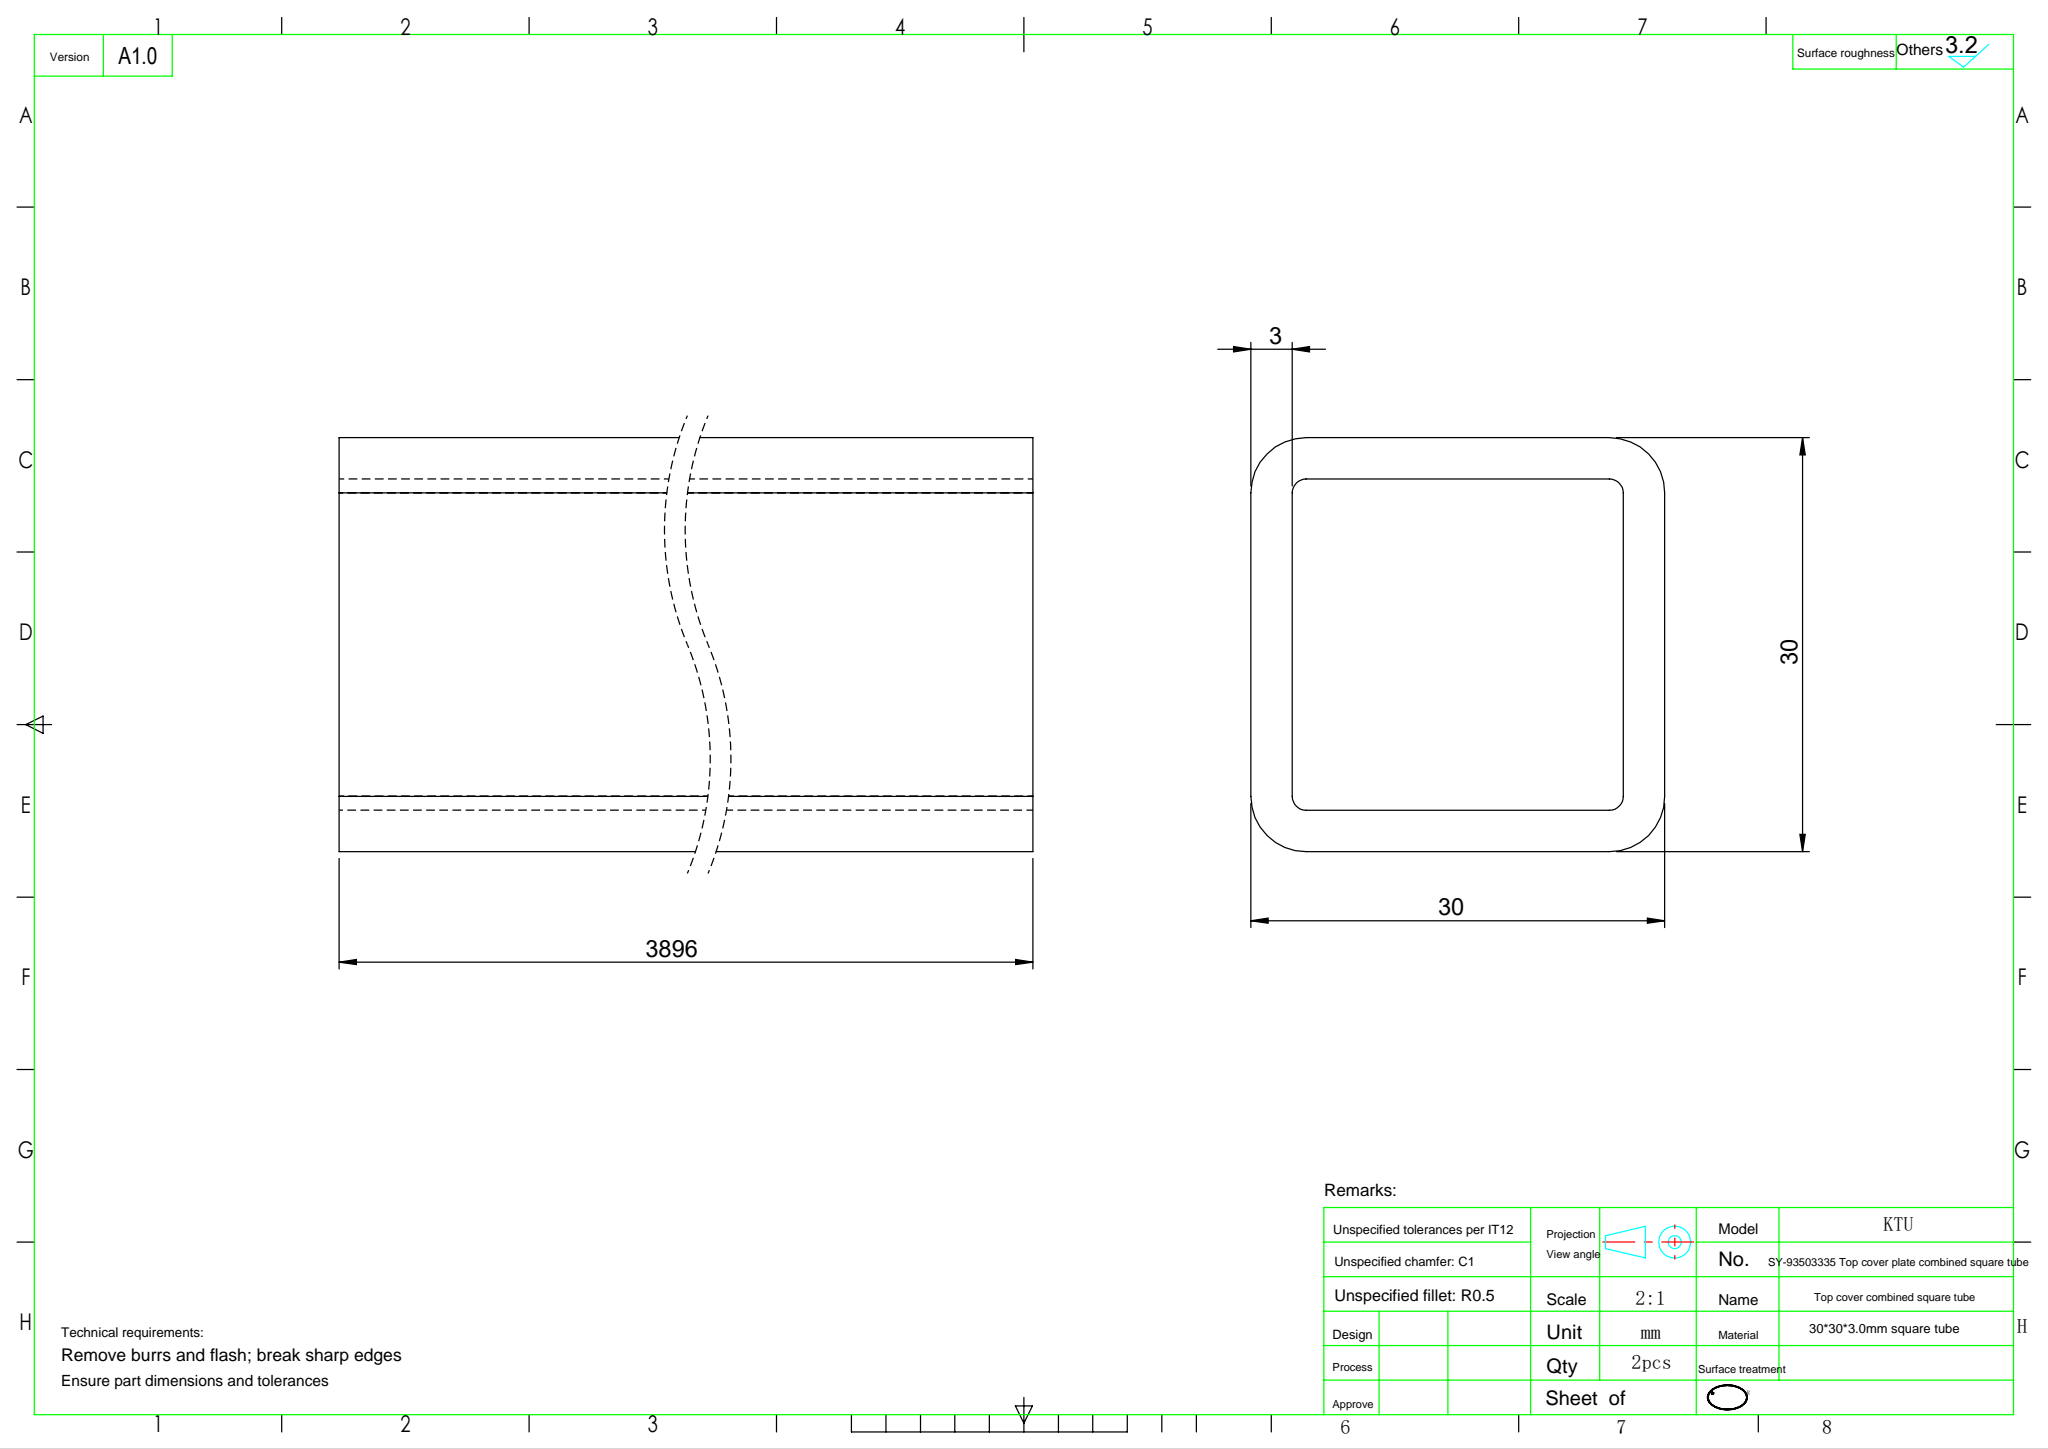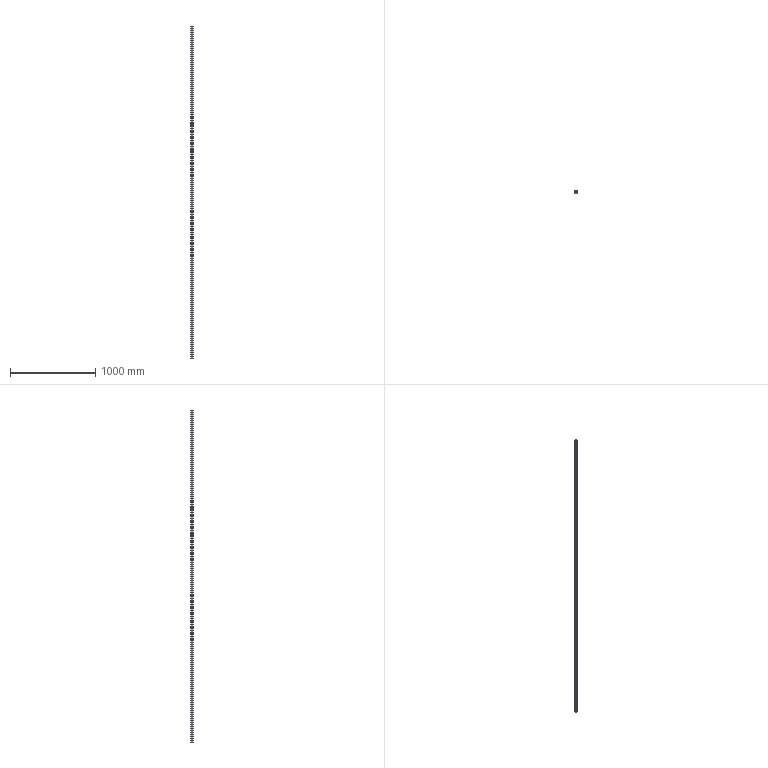Part | SolidWorks | features ExtruThin 1 | 1 solid | 18 faces | box 30 x 30 x 3896 mm | volume 1212139 mm3 | plane 10 | cylinder 8 | commonest cylinder face diameters 2 x4 8 x4
STEP:
#1=CARTESIAN_POINT('',(15.,11.,1948.));
#2=VERTEX_POINT('',#1);
#3=CARTESIAN_POINT('',(11.,15.,1948.));
#4=VERTEX_POINT('',#3);
#5=CARTESIAN_POINT('',(11.,11.,1948.));
#6=DIRECTION('',(0.,0.,1.));
#7=DIRECTION('',(-1.,0.,0.));
#8=AXIS2_PLACEMENT_3D('',#5,#6,#7);
#9=CIRCLE('',#8,4.);
#10=EDGE_CURVE('',#2,#4,#9,.T.);
#11=ORIENTED_EDGE('',*,*,#10,.T.);
#12=CARTESIAN_POINT('',(-11.,15.,1948.));
#13=VERTEX_POINT('',#12);
#14=CARTESIAN_POINT('',(-11.,15.,1948.));
#15=DIRECTION('',(-1.,0.,0.));
#16=VECTOR('',#15,1000.);
#17=LINE('',#14,#16);
#18=EDGE_CURVE('',#4,#13,#17,.T.);
#19=ORIENTED_EDGE('',*,*,#18,.T.);
#20=CARTESIAN_POINT('',(-15.,11.,1948.));
#21=VERTEX_POINT('',#20);
#22=CARTESIAN_POINT('',(-11.,11.,1948.));
#23=DIRECTION('',(0.,0.,1.));
#24=DIRECTION('',(1.,0.,0.));
#25=AXIS2_PLACEMENT_3D('',#22,#23,#24);
#26=CIRCLE('',#25,4.);
#27=EDGE_CURVE('',#13,#21,#26,.T.);
#28=ORIENTED_EDGE('',*,*,#27,.T.);
#29=CARTESIAN_POINT('',(-15.,-11.,1948.));
#30=VERTEX_POINT('',#29);
#31=CARTESIAN_POINT('',(-15.,11.,1948.));
#32=DIRECTION('',(0.,-1.,0.));
#33=VECTOR('',#32,1000.);
#34=LINE('',#31,#33);
#35=EDGE_CURVE('',#21,#30,#34,.T.);
#36=ORIENTED_EDGE('',*,*,#35,.T.);
#37=CARTESIAN_POINT('',(-11.,-15.,1948.));
#38=VERTEX_POINT('',#37);
#39=CARTESIAN_POINT('',(-11.,-11.,1948.));
#40=DIRECTION('',(0.,0.,1.));
#41=DIRECTION('',(1.,0.,0.));
#42=AXIS2_PLACEMENT_3D('',#39,#40,#41);
#43=CIRCLE('',#42,4.);
#44=EDGE_CURVE('',#30,#38,#43,.T.);
#45=ORIENTED_EDGE('',*,*,#44,.T.);
#46=CARTESIAN_POINT('',(11.,-15.,1948.));
#47=VERTEX_POINT('',#46);
#48=CARTESIAN_POINT('',(-11.,-15.,1948.));
#49=DIRECTION('',(1.,0.,0.));
#50=VECTOR('',#49,1000.);
#51=LINE('',#48,#50);
#52=EDGE_CURVE('',#38,#47,#51,.T.);
#53=ORIENTED_EDGE('',*,*,#52,.T.);
#54=CARTESIAN_POINT('',(15.,-11.,1948.));
#55=VERTEX_POINT('',#54);
#56=CARTESIAN_POINT('',(11.,-11.,1948.));
#57=DIRECTION('',(0.,0.,1.));
#58=DIRECTION('',(1.,0.,0.));
#59=AXIS2_PLACEMENT_3D('',#56,#57,#58);
#60=CIRCLE('',#59,4.);
#61=EDGE_CURVE('',#47,#55,#60,.T.);
#62=ORIENTED_EDGE('',*,*,#61,.T.);
#63=CARTESIAN_POINT('',(15.,11.,1948.));
#64=DIRECTION('',(0.,1.,0.));
#65=VECTOR('',#64,1000.);
#66=LINE('',#63,#65);
#67=EDGE_CURVE('',#55,#2,#66,.T.);
#68=ORIENTED_EDGE('',*,*,#67,.T.);
#69=EDGE_LOOP('',(#11,#19,#28,#36,#45,#53,#62,#68));
#70=FACE_OUTER_BOUND('',#69,.T.);
#71=CARTESIAN_POINT('',(11.,12.,1948.));
#72=VERTEX_POINT('',#71);
#73=CARTESIAN_POINT('',(-11.,12.,1948.));
#74=VERTEX_POINT('',#73);
#75=CARTESIAN_POINT('',(11.,12.,1948.));
#76=DIRECTION('',(-1.,0.,0.));
#77=VECTOR('',#76,1000.);
#78=LINE('',#75,#77);
#79=EDGE_CURVE('',#72,#74,#78,.T.);
#80=ORIENTED_EDGE('',*,*,#79,.F.);
#81=CARTESIAN_POINT('',(12.,11.,1948.));
#82=VERTEX_POINT('',#81);
#83=CARTESIAN_POINT('',(11.,11.,1948.));
#84=DIRECTION('',(0.,0.,1.));
#85=DIRECTION('',(-1.,0.,0.));
#86=AXIS2_PLACEMENT_3D('',#83,#84,#85);
#87=CIRCLE('',#86,1.);
#88=EDGE_CURVE('',#82,#72,#87,.T.);
#89=ORIENTED_EDGE('',*,*,#88,.F.);
#90=CARTESIAN_POINT('',(12.,-11.,1948.));
#91=VERTEX_POINT('',#90);
#92=CARTESIAN_POINT('',(12.,11.,1948.));
#93=DIRECTION('',(0.,1.,0.));
#94=VECTOR('',#93,1000.);
#95=LINE('',#92,#94);
#96=EDGE_CURVE('',#91,#82,#95,.T.);
#97=ORIENTED_EDGE('',*,*,#96,.F.);
#98=CARTESIAN_POINT('',(11.,-12.,1948.));
#99=VERTEX_POINT('',#98);
#100=CARTESIAN_POINT('',(11.,-11.,1948.));
#101=DIRECTION('',(0.,0.,1.));
#102=DIRECTION('',(-1.,0.,0.));
#103=AXIS2_PLACEMENT_3D('',#100,#101,#102);
#104=CIRCLE('',#103,1.);
#105=EDGE_CURVE('',#99,#91,#104,.T.);
#106=ORIENTED_EDGE('',*,*,#105,.F.);
#107=CARTESIAN_POINT('',(-11.,-12.,1948.));
#108=VERTEX_POINT('',#107);
#109=CARTESIAN_POINT('',(11.,-12.,1948.));
#110=DIRECTION('',(1.,0.,0.));
#111=VECTOR('',#110,1000.);
#112=LINE('',#109,#111);
#113=EDGE_CURVE('',#108,#99,#112,.T.);
#114=ORIENTED_EDGE('',*,*,#113,.F.);
#115=CARTESIAN_POINT('',(-12.,-11.,1948.));
#116=VERTEX_POINT('',#115);
#117=CARTESIAN_POINT('',(-11.,-11.,1948.));
#118=DIRECTION('',(0.,0.,1.));
#119=DIRECTION('',(-1.,0.,0.));
#120=AXIS2_PLACEMENT_3D('',#117,#118,#119);
#121=CIRCLE('',#120,1.);
#122=EDGE_CURVE('',#116,#108,#121,.T.);
#123=ORIENTED_EDGE('',*,*,#122,.F.);
#124=CARTESIAN_POINT('',(-12.,11.,1948.));
#125=VERTEX_POINT('',#124);
#126=CARTESIAN_POINT('',(-12.,11.,1948.));
#127=DIRECTION('',(0.,-1.,0.));
#128=VECTOR('',#127,1000.);
#129=LINE('',#126,#128);
#130=EDGE_CURVE('',#125,#116,#129,.T.);
#131=ORIENTED_EDGE('',*,*,#130,.F.);
#132=CARTESIAN_POINT('',(-11.,11.,1948.));
#133=DIRECTION('',(0.,0.,1.));
#134=DIRECTION('',(-1.,0.,0.));
#135=AXIS2_PLACEMENT_3D('',#132,#133,#134);
#136=CIRCLE('',#135,1.);
#137=EDGE_CURVE('',#74,#125,#136,.T.);
#138=ORIENTED_EDGE('',*,*,#137,.F.);
#139=EDGE_LOOP('',(#80,#89,#97,#106,#114,#123,#131,#138));
#140=FACE_BOUND('',#139,.T.);
#141=CARTESIAN_POINT('',(11.,11.,1948.));
#142=DIRECTION('',(0.,0.,1.));
#143=DIRECTION('',(1.,0.,0.));
#144=AXIS2_PLACEMENT_3D('',#141,#142,#143);
#145=PLANE('',#144);
#146=ADVANCED_FACE('',(#70,#140),#145,.T.);
#147=CARTESIAN_POINT('',(15.,11.,-1948.));
#148=VERTEX_POINT('',#147);
#149=CARTESIAN_POINT('',(11.,15.,-1948.));
#150=VERTEX_POINT('',#149);
#151=CARTESIAN_POINT('',(11.,11.,-1948.));
#152=DIRECTION('',(0.,0.,1.));
#153=DIRECTION('',(-1.,0.,0.));
#154=AXIS2_PLACEMENT_3D('',#151,#152,#153);
#155=CIRCLE('',#154,4.);
#156=EDGE_CURVE('',#148,#150,#155,.T.);
#157=ORIENTED_EDGE('',*,*,#156,.F.);
#158=CARTESIAN_POINT('',(15.,-11.,-1948.));
#159=VERTEX_POINT('',#158);
#160=CARTESIAN_POINT('',(15.,11.,-1948.));
#161=DIRECTION('',(0.,1.,0.));
#162=VECTOR('',#161,1000.);
#163=LINE('',#160,#162);
#164=EDGE_CURVE('',#159,#148,#163,.T.);
#165=ORIENTED_EDGE('',*,*,#164,.F.);
#166=CARTESIAN_POINT('',(11.,-15.,-1948.));
#167=VERTEX_POINT('',#166);
#168=CARTESIAN_POINT('',(11.,-11.,-1948.));
#169=DIRECTION('',(0.,0.,1.));
#170=DIRECTION('',(1.,0.,0.));
#171=AXIS2_PLACEMENT_3D('',#168,#169,#170);
#172=CIRCLE('',#171,4.);
#173=EDGE_CURVE('',#167,#159,#172,.T.);
#174=ORIENTED_EDGE('',*,*,#173,.F.);
#175=CARTESIAN_POINT('',(-11.,-15.,-1948.));
#176=VERTEX_POINT('',#175);
#177=CARTESIAN_POINT('',(-11.,-15.,-1948.));
#178=DIRECTION('',(1.,0.,0.));
#179=VECTOR('',#178,1000.);
#180=LINE('',#177,#179);
#181=EDGE_CURVE('',#176,#167,#180,.T.);
#182=ORIENTED_EDGE('',*,*,#181,.F.);
#183=CARTESIAN_POINT('',(-15.,-11.,-1948.));
#184=VERTEX_POINT('',#183);
#185=CARTESIAN_POINT('',(-11.,-11.,-1948.));
#186=DIRECTION('',(0.,0.,1.));
#187=DIRECTION('',(1.,0.,0.));
#188=AXIS2_PLACEMENT_3D('',#185,#186,#187);
#189=CIRCLE('',#188,4.);
#190=EDGE_CURVE('',#184,#176,#189,.T.);
#191=ORIENTED_EDGE('',*,*,#190,.F.);
#192=CARTESIAN_POINT('',(-15.,11.,-1948.));
#193=VERTEX_POINT('',#192);
#194=CARTESIAN_POINT('',(-15.,11.,-1948.));
#195=DIRECTION('',(0.,-1.,0.));
#196=VECTOR('',#195,1000.);
#197=LINE('',#194,#196);
#198=EDGE_CURVE('',#193,#184,#197,.T.);
#199=ORIENTED_EDGE('',*,*,#198,.F.);
#200=CARTESIAN_POINT('',(-11.,15.,-1948.));
#201=VERTEX_POINT('',#200);
#202=CARTESIAN_POINT('',(-11.,11.,-1948.));
#203=DIRECTION('',(0.,0.,1.));
#204=DIRECTION('',(1.,0.,0.));
#205=AXIS2_PLACEMENT_3D('',#202,#203,#204);
#206=CIRCLE('',#205,4.);
#207=EDGE_CURVE('',#201,#193,#206,.T.);
#208=ORIENTED_EDGE('',*,*,#207,.F.);
#209=CARTESIAN_POINT('',(-11.,15.,-1948.));
#210=DIRECTION('',(-1.,0.,0.));
#211=VECTOR('',#210,1000.);
#212=LINE('',#209,#211);
#213=EDGE_CURVE('',#150,#201,#212,.T.);
#214=ORIENTED_EDGE('',*,*,#213,.F.);
#215=EDGE_LOOP('',(#157,#165,#174,#182,#191,#199,#208,#214));
#216=FACE_OUTER_BOUND('',#215,.T.);
#217=CARTESIAN_POINT('',(12.,11.,-1948.));
#218=VERTEX_POINT('',#217);
#219=CARTESIAN_POINT('',(11.,12.,-1948.));
#220=VERTEX_POINT('',#219);
#221=CARTESIAN_POINT('',(11.,11.,-1948.));
#222=DIRECTION('',(0.,0.,1.));
#223=DIRECTION('',(-1.,0.,0.));
#224=AXIS2_PLACEMENT_3D('',#221,#222,#223);
#225=CIRCLE('',#224,1.);
#226=EDGE_CURVE('',#218,#220,#225,.T.);
#227=ORIENTED_EDGE('',*,*,#226,.T.);
#228=CARTESIAN_POINT('',(-11.,12.,-1948.));
#229=VERTEX_POINT('',#228);
#230=CARTESIAN_POINT('',(11.,12.,-1948.));
#231=DIRECTION('',(-1.,0.,0.));
#232=VECTOR('',#231,1000.);
#233=LINE('',#230,#232);
#234=EDGE_CURVE('',#220,#229,#233,.T.);
#235=ORIENTED_EDGE('',*,*,#234,.T.);
#236=CARTESIAN_POINT('',(-12.,11.,-1948.));
#237=VERTEX_POINT('',#236);
#238=CARTESIAN_POINT('',(-11.,11.,-1948.));
#239=DIRECTION('',(0.,0.,1.));
#240=DIRECTION('',(-1.,0.,0.));
#241=AXIS2_PLACEMENT_3D('',#238,#239,#240);
#242=CIRCLE('',#241,1.);
#243=EDGE_CURVE('',#229,#237,#242,.T.);
#244=ORIENTED_EDGE('',*,*,#243,.T.);
#245=CARTESIAN_POINT('',(-12.,-11.,-1948.));
#246=VERTEX_POINT('',#245);
#247=CARTESIAN_POINT('',(-12.,11.,-1948.));
#248=DIRECTION('',(0.,-1.,0.));
#249=VECTOR('',#248,1000.);
#250=LINE('',#247,#249);
#251=EDGE_CURVE('',#237,#246,#250,.T.);
#252=ORIENTED_EDGE('',*,*,#251,.T.);
#253=CARTESIAN_POINT('',(-11.,-12.,-1948.));
#254=VERTEX_POINT('',#253);
#255=CARTESIAN_POINT('',(-11.,-11.,-1948.));
#256=DIRECTION('',(0.,0.,1.));
#257=DIRECTION('',(-1.,0.,0.));
#258=AXIS2_PLACEMENT_3D('',#255,#256,#257);
#259=CIRCLE('',#258,1.);
#260=EDGE_CURVE('',#246,#254,#259,.T.);
#261=ORIENTED_EDGE('',*,*,#260,.T.);
#262=CARTESIAN_POINT('',(11.,-12.,-1948.));
#263=VERTEX_POINT('',#262);
#264=CARTESIAN_POINT('',(11.,-12.,-1948.));
#265=DIRECTION('',(1.,0.,0.));
#266=VECTOR('',#265,1000.);
#267=LINE('',#264,#266);
#268=EDGE_CURVE('',#254,#263,#267,.T.);
#269=ORIENTED_EDGE('',*,*,#268,.T.);
#270=CARTESIAN_POINT('',(12.,-11.,-1948.));
#271=VERTEX_POINT('',#270);
#272=CARTESIAN_POINT('',(11.,-11.,-1948.));
#273=DIRECTION('',(0.,0.,1.));
#274=DIRECTION('',(-1.,0.,0.));
#275=AXIS2_PLACEMENT_3D('',#272,#273,#274);
#276=CIRCLE('',#275,1.);
#277=EDGE_CURVE('',#263,#271,#276,.T.);
#278=ORIENTED_EDGE('',*,*,#277,.T.);
#279=CARTESIAN_POINT('',(12.,11.,-1948.));
#280=DIRECTION('',(0.,1.,0.));
#281=VECTOR('',#280,1000.);
#282=LINE('',#279,#281);
#283=EDGE_CURVE('',#271,#218,#282,.T.);
#284=ORIENTED_EDGE('',*,*,#283,.T.);
#285=EDGE_LOOP('',(#227,#235,#244,#252,#261,#269,#278,#284));
#286=FACE_BOUND('',#285,.T.);
#287=CARTESIAN_POINT('',(11.,11.,-1948.));
#288=DIRECTION('',(0.,0.,1.));
#289=DIRECTION('',(1.,0.,0.));
#290=AXIS2_PLACEMENT_3D('',#287,#288,#289);
#291=PLANE('',#290);
#292=ADVANCED_FACE('',(#216,#286),#291,.F.);
#293=ORIENTED_EDGE('',*,*,#156,.T.);
#294=CARTESIAN_POINT('',(11.,15.,1948.));
#295=DIRECTION('',(0.,0.,-1.));
#296=VECTOR('',#295,1000.);
#297=LINE('',#294,#296);
#298=EDGE_CURVE('',#4,#150,#297,.T.);
#299=ORIENTED_EDGE('',*,*,#298,.F.);
#300=ORIENTED_EDGE('',*,*,#10,.F.);
#301=CARTESIAN_POINT('',(15.,11.,1948.));
#302=DIRECTION('',(0.,0.,-1.));
#303=VECTOR('',#302,1000.);
#304=LINE('',#301,#303);
#305=EDGE_CURVE('',#2,#148,#304,.T.);
#306=ORIENTED_EDGE('',*,*,#305,.T.);
#307=EDGE_LOOP('',(#293,#299,#300,#306));
#308=FACE_OUTER_BOUND('',#307,.T.);
#309=CARTESIAN_POINT('',(11.,11.,1948.));
#310=DIRECTION('',(0.,0.,-1.));
#311=DIRECTION('',(-1.,0.,0.));
#312=AXIS2_PLACEMENT_3D('',#309,#310,#311);
#313=CYLINDRICAL_SURFACE('',#312,4.);
#314=ADVANCED_FACE('',(#308),#313,.T.);
#315=ORIENTED_EDGE('',*,*,#213,.T.);
#316=CARTESIAN_POINT('',(-11.,15.,1948.));
#317=DIRECTION('',(0.,0.,-1.));
#318=VECTOR('',#317,1000.);
#319=LINE('',#316,#318);
#320=EDGE_CURVE('',#13,#201,#319,.T.);
#321=ORIENTED_EDGE('',*,*,#320,.F.);
#322=ORIENTED_EDGE('',*,*,#18,.F.);
#323=ORIENTED_EDGE('',*,*,#298,.T.);
#324=EDGE_LOOP('',(#315,#321,#322,#323));
#325=FACE_OUTER_BOUND('',#324,.T.);
#326=CARTESIAN_POINT('',(-11.,15.,1948.));
#327=DIRECTION('',(0.,-1.,0.));
#328=DIRECTION('',(0.,0.,-1.));
#329=AXIS2_PLACEMENT_3D('',#326,#327,#328);
#330=PLANE('',#329);
#331=ADVANCED_FACE('',(#325),#330,.F.);
#332=ORIENTED_EDGE('',*,*,#207,.T.);
#333=CARTESIAN_POINT('',(-15.,11.,1948.));
#334=DIRECTION('',(0.,0.,-1.));
#335=VECTOR('',#334,1000.);
#336=LINE('',#333,#335);
#337=EDGE_CURVE('',#21,#193,#336,.T.);
#338=ORIENTED_EDGE('',*,*,#337,.F.);
#339=ORIENTED_EDGE('',*,*,#27,.F.);
#340=ORIENTED_EDGE('',*,*,#320,.T.);
#341=EDGE_LOOP('',(#332,#338,#339,#340));
#342=FACE_OUTER_BOUND('',#341,.T.);
#343=CARTESIAN_POINT('',(-11.,11.,1948.));
#344=DIRECTION('',(0.,0.,-1.));
#345=DIRECTION('',(-1.,0.,0.));
#346=AXIS2_PLACEMENT_3D('',#343,#344,#345);
#347=CYLINDRICAL_SURFACE('',#346,4.);
#348=ADVANCED_FACE('',(#342),#347,.T.);
#349=ORIENTED_EDGE('',*,*,#198,.T.);
#350=CARTESIAN_POINT('',(-15.,-11.,1948.));
#351=DIRECTION('',(0.,0.,-1.));
#352=VECTOR('',#351,1000.);
#353=LINE('',#350,#352);
#354=EDGE_CURVE('',#30,#184,#353,.T.);
#355=ORIENTED_EDGE('',*,*,#354,.F.);
#356=ORIENTED_EDGE('',*,*,#35,.F.);
#357=ORIENTED_EDGE('',*,*,#337,.T.);
#358=EDGE_LOOP('',(#349,#355,#356,#357));
#359=FACE_OUTER_BOUND('',#358,.T.);
#360=CARTESIAN_POINT('',(-15.,11.,1948.));
#361=DIRECTION('',(1.,0.,0.));
#362=DIRECTION('',(0.,1.,0.));
#363=AXIS2_PLACEMENT_3D('',#360,#361,#362);
#364=PLANE('',#363);
#365=ADVANCED_FACE('',(#359),#364,.F.);
#366=ORIENTED_EDGE('',*,*,#190,.T.);
#367=CARTESIAN_POINT('',(-11.,-15.,1948.));
#368=DIRECTION('',(0.,0.,-1.));
#369=VECTOR('',#368,1000.);
#370=LINE('',#367,#369);
#371=EDGE_CURVE('',#38,#176,#370,.T.);
#372=ORIENTED_EDGE('',*,*,#371,.F.);
#373=ORIENTED_EDGE('',*,*,#44,.F.);
#374=ORIENTED_EDGE('',*,*,#354,.T.);
#375=EDGE_LOOP('',(#366,#372,#373,#374));
#376=FACE_OUTER_BOUND('',#375,.T.);
#377=CARTESIAN_POINT('',(-11.,-11.,1948.));
#378=DIRECTION('',(0.,0.,-1.));
#379=DIRECTION('',(-1.,0.,0.));
#380=AXIS2_PLACEMENT_3D('',#377,#378,#379);
#381=CYLINDRICAL_SURFACE('',#380,4.);
#382=ADVANCED_FACE('',(#376),#381,.T.);
#383=ORIENTED_EDGE('',*,*,#181,.T.);
#384=CARTESIAN_POINT('',(11.,-15.,1948.));
#385=DIRECTION('',(0.,0.,-1.));
#386=VECTOR('',#385,1000.);
#387=LINE('',#384,#386);
#388=EDGE_CURVE('',#47,#167,#387,.T.);
#389=ORIENTED_EDGE('',*,*,#388,.F.);
#390=ORIENTED_EDGE('',*,*,#52,.F.);
#391=ORIENTED_EDGE('',*,*,#371,.T.);
#392=EDGE_LOOP('',(#383,#389,#390,#391));
#393=FACE_OUTER_BOUND('',#392,.T.);
#394=CARTESIAN_POINT('',(-11.,-15.,1948.));
#395=DIRECTION('',(0.,1.,0.));
#396=DIRECTION('',(0.,0.,1.));
#397=AXIS2_PLACEMENT_3D('',#394,#395,#396);
#398=PLANE('',#397);
#399=ADVANCED_FACE('',(#393),#398,.F.);
#400=ORIENTED_EDGE('',*,*,#173,.T.);
#401=CARTESIAN_POINT('',(15.,-11.,1948.));
#402=DIRECTION('',(0.,0.,-1.));
#403=VECTOR('',#402,1000.);
#404=LINE('',#401,#403);
#405=EDGE_CURVE('',#55,#159,#404,.T.);
#406=ORIENTED_EDGE('',*,*,#405,.F.);
#407=ORIENTED_EDGE('',*,*,#61,.F.);
#408=ORIENTED_EDGE('',*,*,#388,.T.);
#409=EDGE_LOOP('',(#400,#406,#407,#408));
#410=FACE_OUTER_BOUND('',#409,.T.);
#411=CARTESIAN_POINT('',(11.,-11.,1948.));
#412=DIRECTION('',(0.,0.,-1.));
#413=DIRECTION('',(-1.,0.,0.));
#414=AXIS2_PLACEMENT_3D('',#411,#412,#413);
#415=CYLINDRICAL_SURFACE('',#414,4.);
#416=ADVANCED_FACE('',(#410),#415,.T.);
#417=ORIENTED_EDGE('',*,*,#164,.T.);
#418=ORIENTED_EDGE('',*,*,#305,.F.);
#419=ORIENTED_EDGE('',*,*,#67,.F.);
#420=ORIENTED_EDGE('',*,*,#405,.T.);
#421=EDGE_LOOP('',(#417,#418,#419,#420));
#422=FACE_OUTER_BOUND('',#421,.T.);
#423=CARTESIAN_POINT('',(15.,11.,1948.));
#424=DIRECTION('',(-1.,0.,0.));
#425=DIRECTION('',(0.,-1.,0.));
#426=AXIS2_PLACEMENT_3D('',#423,#424,#425);
#427=PLANE('',#426);
#428=ADVANCED_FACE('',(#422),#427,.F.);
#429=ORIENTED_EDGE('',*,*,#226,.F.);
#430=CARTESIAN_POINT('',(12.,11.,1948.));
#431=DIRECTION('',(0.,0.,-1.));
#432=VECTOR('',#431,1000.);
#433=LINE('',#430,#432);
#434=EDGE_CURVE('',#82,#218,#433,.T.);
#435=ORIENTED_EDGE('',*,*,#434,.F.);
#436=ORIENTED_EDGE('',*,*,#88,.T.);
#437=CARTESIAN_POINT('',(11.,12.,1948.));
#438=DIRECTION('',(0.,0.,-1.));
#439=VECTOR('',#438,1000.);
#440=LINE('',#437,#439);
#441=EDGE_CURVE('',#72,#220,#440,.T.);
#442=ORIENTED_EDGE('',*,*,#441,.T.);
#443=EDGE_LOOP('',(#429,#435,#436,#442));
#444=FACE_OUTER_BOUND('',#443,.T.);
#445=CARTESIAN_POINT('',(11.,11.,1948.));
#446=DIRECTION('',(0.,0.,-1.));
#447=DIRECTION('',(-1.,0.,0.));
#448=AXIS2_PLACEMENT_3D('',#445,#446,#447);
#449=CYLINDRICAL_SURFACE('',#448,1.);
#450=ADVANCED_FACE('',(#444),#449,.F.);
#451=ORIENTED_EDGE('',*,*,#234,.F.);
#452=ORIENTED_EDGE('',*,*,#441,.F.);
#453=ORIENTED_EDGE('',*,*,#79,.T.);
#454=CARTESIAN_POINT('',(-11.,12.,1948.));
#455=DIRECTION('',(0.,0.,-1.));
#456=VECTOR('',#455,1000.);
#457=LINE('',#454,#456);
#458=EDGE_CURVE('',#74,#229,#457,.T.);
#459=ORIENTED_EDGE('',*,*,#458,.T.);
#460=EDGE_LOOP('',(#451,#452,#453,#459));
#461=FACE_OUTER_BOUND('',#460,.T.);
#462=CARTESIAN_POINT('',(11.,12.,1948.));
#463=DIRECTION('',(0.,-1.,0.));
#464=DIRECTION('',(0.,0.,-1.));
#465=AXIS2_PLACEMENT_3D('',#462,#463,#464);
#466=PLANE('',#465);
#467=ADVANCED_FACE('',(#461),#466,.T.);
#468=ORIENTED_EDGE('',*,*,#243,.F.);
#469=ORIENTED_EDGE('',*,*,#458,.F.);
#470=ORIENTED_EDGE('',*,*,#137,.T.);
#471=CARTESIAN_POINT('',(-12.,11.,1948.));
#472=DIRECTION('',(0.,0.,-1.));
#473=VECTOR('',#472,1000.);
#474=LINE('',#471,#473);
#475=EDGE_CURVE('',#125,#237,#474,.T.);
#476=ORIENTED_EDGE('',*,*,#475,.T.);
#477=EDGE_LOOP('',(#468,#469,#470,#476));
#478=FACE_OUTER_BOUND('',#477,.T.);
#479=CARTESIAN_POINT('',(-11.,11.,1948.));
#480=DIRECTION('',(0.,0.,-1.));
#481=DIRECTION('',(-1.,0.,0.));
#482=AXIS2_PLACEMENT_3D('',#479,#480,#481);
#483=CYLINDRICAL_SURFACE('',#482,1.);
#484=ADVANCED_FACE('',(#478),#483,.F.);
#485=ORIENTED_EDGE('',*,*,#251,.F.);
#486=ORIENTED_EDGE('',*,*,#475,.F.);
#487=ORIENTED_EDGE('',*,*,#130,.T.);
#488=CARTESIAN_POINT('',(-12.,-11.,1948.));
#489=DIRECTION('',(0.,0.,-1.));
#490=VECTOR('',#489,1000.);
#491=LINE('',#488,#490);
#492=EDGE_CURVE('',#116,#246,#491,.T.);
#493=ORIENTED_EDGE('',*,*,#492,.T.);
#494=EDGE_LOOP('',(#485,#486,#487,#493));
#495=FACE_OUTER_BOUND('',#494,.T.);
#496=CARTESIAN_POINT('',(-12.,11.,1948.));
#497=DIRECTION('',(1.,0.,0.));
#498=DIRECTION('',(0.,1.,0.));
#499=AXIS2_PLACEMENT_3D('',#496,#497,#498);
#500=PLANE('',#499);
#501=ADVANCED_FACE('',(#495),#500,.T.);
#502=ORIENTED_EDGE('',*,*,#260,.F.);
#503=ORIENTED_EDGE('',*,*,#492,.F.);
#504=ORIENTED_EDGE('',*,*,#122,.T.);
#505=CARTESIAN_POINT('',(-11.,-12.,1948.));
#506=DIRECTION('',(0.,0.,-1.));
#507=VECTOR('',#506,1000.);
#508=LINE('',#505,#507);
#509=EDGE_CURVE('',#108,#254,#508,.T.);
#510=ORIENTED_EDGE('',*,*,#509,.T.);
#511=EDGE_LOOP('',(#502,#503,#504,#510));
#512=FACE_OUTER_BOUND('',#511,.T.);
#513=CARTESIAN_POINT('',(-11.,-11.,1948.));
#514=DIRECTION('',(0.,0.,-1.));
#515=DIRECTION('',(-1.,0.,0.));
#516=AXIS2_PLACEMENT_3D('',#513,#514,#515);
#517=CYLINDRICAL_SURFACE('',#516,1.);
#518=ADVANCED_FACE('',(#512),#517,.F.);
#519=ORIENTED_EDGE('',*,*,#268,.F.);
#520=ORIENTED_EDGE('',*,*,#509,.F.);
#521=ORIENTED_EDGE('',*,*,#113,.T.);
#522=CARTESIAN_POINT('',(11.,-12.,1948.));
#523=DIRECTION('',(0.,0.,-1.));
#524=VECTOR('',#523,1000.);
#525=LINE('',#522,#524);
#526=EDGE_CURVE('',#99,#263,#525,.T.);
#527=ORIENTED_EDGE('',*,*,#526,.T.);
#528=EDGE_LOOP('',(#519,#520,#521,#527));
#529=FACE_OUTER_BOUND('',#528,.T.);
#530=CARTESIAN_POINT('',(11.,-12.,1948.));
#531=DIRECTION('',(0.,1.,0.));
#532=DIRECTION('',(0.,0.,1.));
#533=AXIS2_PLACEMENT_3D('',#530,#531,#532);
#534=PLANE('',#533);
#535=ADVANCED_FACE('',(#529),#534,.T.);
#536=ORIENTED_EDGE('',*,*,#277,.F.);
#537=ORIENTED_EDGE('',*,*,#526,.F.);
#538=ORIENTED_EDGE('',*,*,#105,.T.);
#539=CARTESIAN_POINT('',(12.,-11.,1948.));
#540=DIRECTION('',(0.,0.,-1.));
#541=VECTOR('',#540,1000.);
#542=LINE('',#539,#541);
#543=EDGE_CURVE('',#91,#271,#542,.T.);
#544=ORIENTED_EDGE('',*,*,#543,.T.);
#545=EDGE_LOOP('',(#536,#537,#538,#544));
#546=FACE_OUTER_BOUND('',#545,.T.);
#547=CARTESIAN_POINT('',(11.,-11.,1948.));
#548=DIRECTION('',(0.,0.,-1.));
#549=DIRECTION('',(-1.,0.,0.));
#550=AXIS2_PLACEMENT_3D('',#547,#548,#549);
#551=CYLINDRICAL_SURFACE('',#550,1.);
#552=ADVANCED_FACE('',(#546),#551,.F.);
#553=ORIENTED_EDGE('',*,*,#283,.F.);
#554=ORIENTED_EDGE('',*,*,#543,.F.);
#555=ORIENTED_EDGE('',*,*,#96,.T.);
#556=ORIENTED_EDGE('',*,*,#434,.T.);
#557=EDGE_LOOP('',(#553,#554,#555,#556));
#558=FACE_OUTER_BOUND('',#557,.T.);
#559=CARTESIAN_POINT('',(12.,11.,1948.));
#560=DIRECTION('',(-1.,0.,0.));
#561=DIRECTION('',(0.,-1.,0.));
#562=AXIS2_PLACEMENT_3D('',#559,#560,#561);
#563=PLANE('',#562);
#564=ADVANCED_FACE('',(#558),#563,.T.);
#565=CLOSED_SHELL('',(#146,#292,#314,#331,#348,#365,#382,#399,#416,#428,#450,#467,#484,#501,#518,#535,#552,#564));
#566=MANIFOLD_SOLID_BREP('',#565);
#567=CARTESIAN_POINT('',(0.,0.,0.));
#568=DIRECTION('',(0.,0.,1.));
#569=DIRECTION('',(1.,0.,0.));
#570=AXIS2_PLACEMENT_3D('',#567,#568,#569);
#571=(LENGTH_UNIT()NAMED_UNIT(*)SI_UNIT(.MILLI.,.METRE.));
#572=UNCERTAINTY_MEASURE_WITH_UNIT(LENGTH_MEASURE(0.00001),#571,'','');
#573=(NAMED_UNIT(*)PLANE_ANGLE_UNIT()SI_UNIT($,.RADIAN.));
#574=(NAMED_UNIT(*)SI_UNIT($,.STERADIAN.)SOLID_ANGLE_UNIT());
#575=(GEOMETRIC_REPRESENTATION_CONTEXT(3)GLOBAL_UNCERTAINTY_ASSIGNED_CONTEXT((#572))GLOBAL_UNIT_ASSIGNED_CONTEXT((#571,#573,#574))REPRESENTATION_CONTEXT('',''));
#576=ADVANCED_BREP_SHAPE_REPRESENTATION('',(#566,#570),#575);